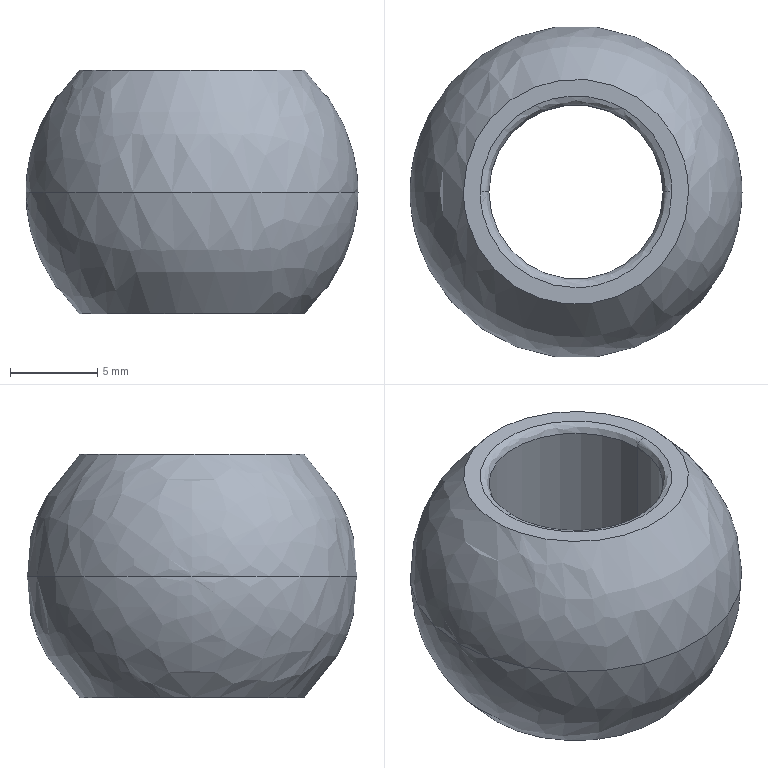Part | STEP file | 0229_Z_PHSC10A_2 | 1 solid | 10 faces | volume 2169 mm3 | spline 6 | cylinder 2 | plane 2 | commonest cylinder face diameters 10 x2